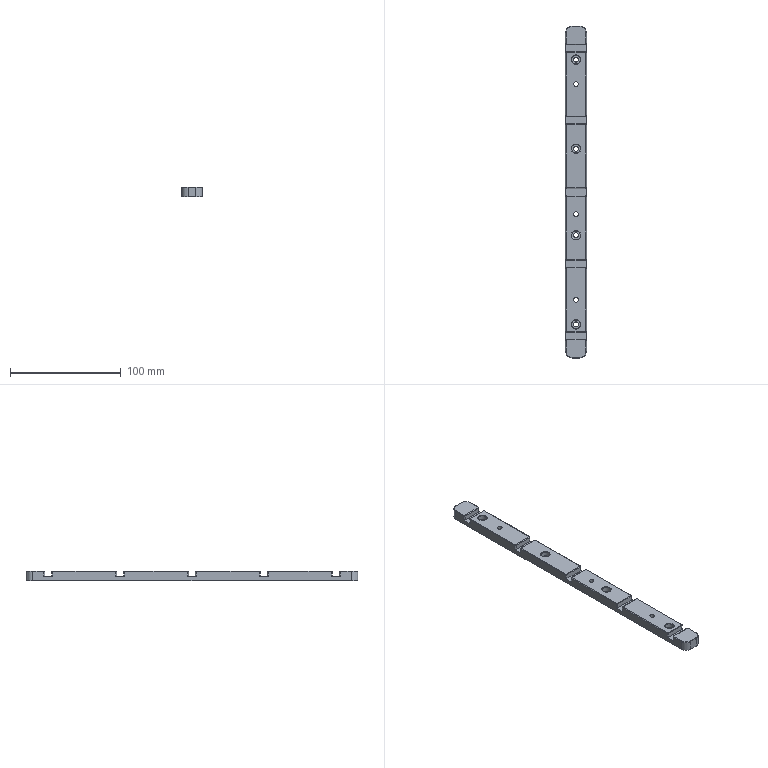Part | 1 solid | 117 faces | box 19 x 300 x 9 mm | volume 46621 mm3 | cylinder 59 | plane 30 | torus 24 | cone 4 | commonest cylinder face diameters 1 x24 2 x20 4.5 x4 7.5 x4 12 x4 4.2 x3